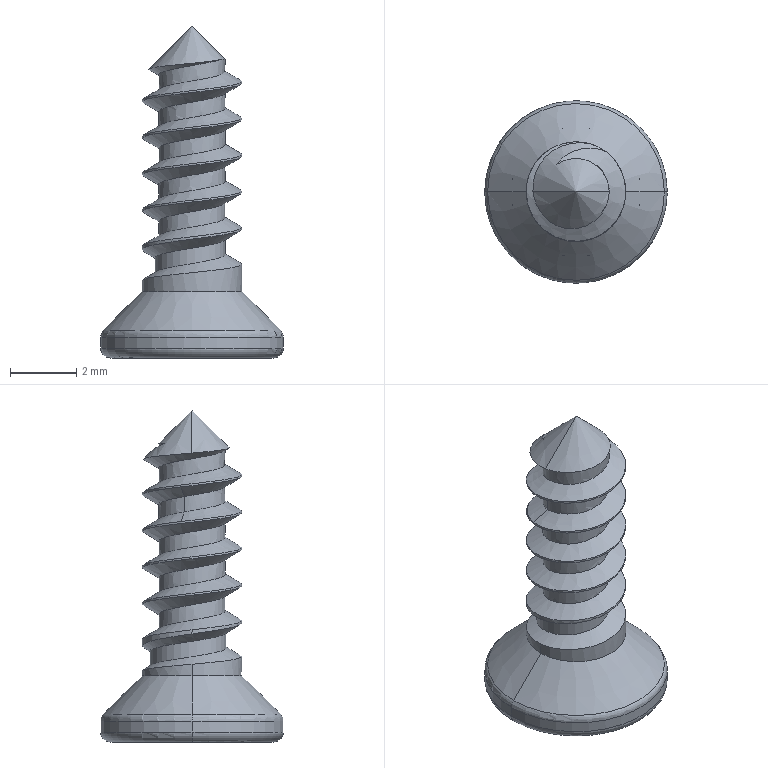Part | NX | features solid 2 | 1 solid | 49 faces | box 5.5 x 5.5 x 10 mm | volume 59.419 mm3 | plane 18 | cylinder 14 | spline 9 | cone 4 | torus 4 | commonest cylinder face diameters 3 x12 5.5 x2